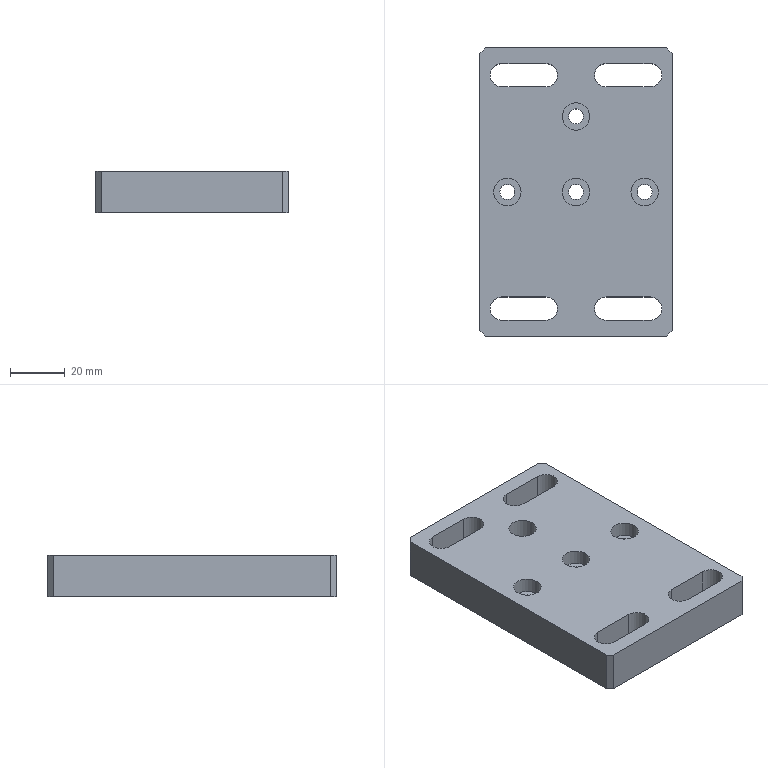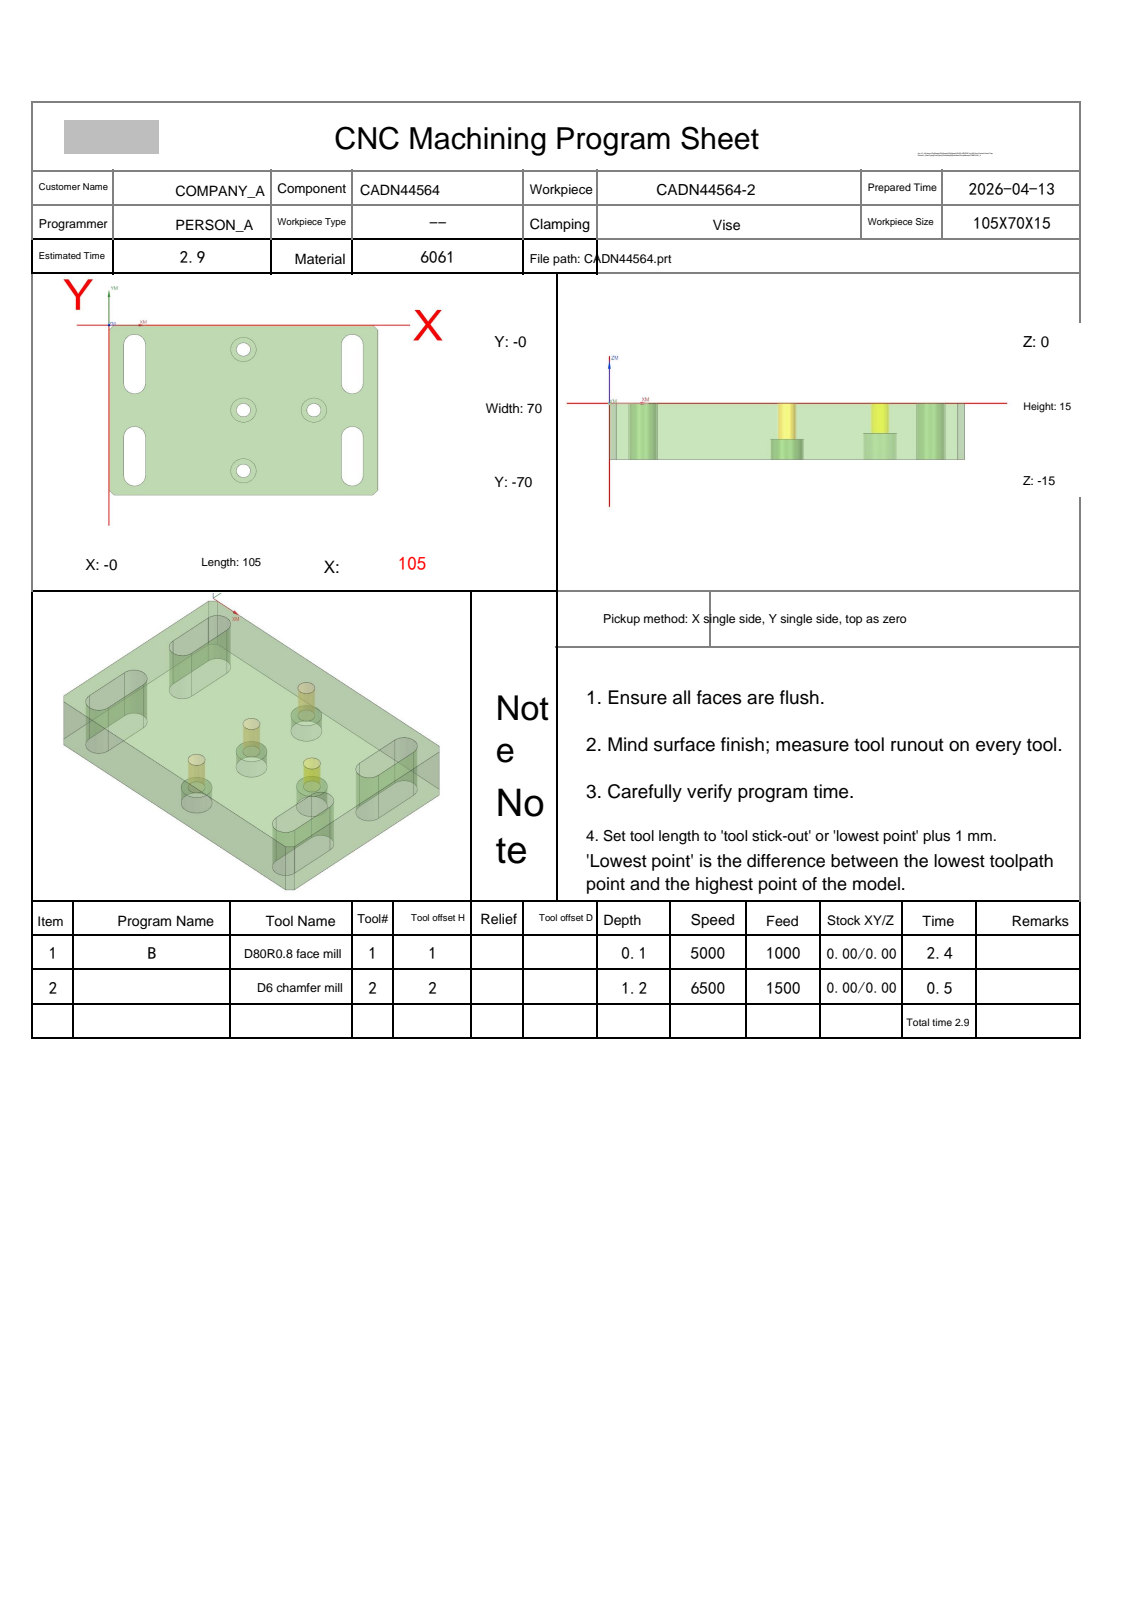NC program | NX | posted by the shop | part box 70 x 105 x 15 mm
Whole program:
%
O0001
(Machine time: 3.19 MIN)
(===Total Tool:2===)
(T1=D80R0.8 face mill D=80.  R=0.8  D-  H01 Z=0.    )
(T2=D6 chamfer mill   D=6.   R=0.   D-  H02 Z=-1.2  )
G80 G90 G17 G49 G40
G91 G28 Z0
M01
N1 T01 M06
(D80R0.8 face mill  D=80. R=0.8 H=01 ce=0.00 di=0.10)
G00 G90 G54 X-45. Y-35. M03 S5000
G43 H01 Z20.
M08
Z6.51
G01 Z4.51 F1000.
X-40.
X145.
X150.
Z6.51
G00 Z8.
X-45.
Z6.02
G01 Z4.02
X-40.
X145.
X150.
Z6.02
G00 Z7.51
X-45.
Z5.53
G01 Z3.53
X-40.
X145.
X150.
Z5.53
G00 Z7.02
X-45.
Z5.04
G01 Z3.04
X-40.
X145.
X150.
Z5.04
G00 Z6.53
X-45.
Z4.55
G01 Z2.55
X-40.
X145.
X150.
Z4.55
G00 Z6.04
X-45.
Z4.06
G01 Z2.06
X-40.
X145.
X150.
Z4.06
G00 Z5.55
X-45.
Z3.57
G01 Z1.57
X-40.
X145.
X150.
Z3.57
G00 Z5.06
X-45.
Z3.08
G01 Z1.08
X-40.
X145.
X150.
Z3.08
G00 Z4.57
X-45.
Z2.59
G01 Z.59
X-40.
X145.
X150.
Z2.59
G00 Z4.08
X-45.
Z2.1
G01 Z.1
X-40.
X145.
X150.
Z2.1
G00 Z20.
G00 G90 X-45. Y-35. M03 S5000
Z20.
Z2.
G01 Z0.0 F1000.
X-40.
X145.
X150.
Z2.
G00 Z20.
G91 G28 Z0.0
M05
M09
G91 G28 Z0.0
M01
N2 T02 M06
(D6 chamfer mill  D=6. R=0. H=02 ce=0.00 di=0.00)
G00 G90 G54 X52.114 Y1.227 M03 S6500
G43 H02 Z20.
M08
Z.172
G01 Z-1.2 F1500.
G03 X52.4 Y1.027 I1.286 J1.532
G01 X52.446 Y.997
X52.5 Y1.
X103.
X103.259 Y.966
X103.5 Y.866
X103.707 Y.707
X105.707 Y-1.293
X105.866 Y-1.5
X105.966 Y-1.741
X106. Y-2.
Y-68.
X105.966 Y-68.259
X105.866 Y-68.5
X105.707 Y-68.707
X103.707 Y-70.707
X103.5 Y-70.866
X103.259 Y-70.966
X103. Y-71.
X2.
X1.741 Y-70.966
X1.5 Y-70.866
X1.293 Y-70.707
X-.707 Y-68.707
X-.866 Y-68.5
X-.966 Y-68.259
X-1. Y-68.
Y-2.
X-.966 Y-1.741
X-.866 Y-1.5
X-.707 Y-1.293
X1.293 Y.707
X1.5 Y.866
X1.741 Y.966
X2. Y1.
X52.5
X52.554 Y.997
X52.6 Y1.027
G03 X52.886 Y1.227 I-1. J1.732
G01 Z.172
G00 Z10.
X91.977 Y-53.614
Z.172
G01 Z-1.2
G03 X91.777 Y-53.9 I1.532 J-1.286
G01 X91.747 Y-53.946
X91.75 Y-54.
Y-62.
G03 X95. Y-65.25 I3.25 J0.0
X98.25 Y-62. I0.0 J3.25
G01 Y-46.
G03 X95. Y-42.75 I-3.25 J0.0
X91.75 Y-46. I0.0 J-3.25
G01 Y-54.
X91.747 Y-54.054
X91.777 Y-54.1
G03 X91.977 Y-54.386 I1.732 J1.
G01 Z.172
G00 Z10.
X79.593 Y-36.565
Z.27
G01 Z-1.2
G03 X79.898 Y-36.734 I1.118 J1.658
G01 X79.946 Y-36.759
X80. Y-36.75
G03 X81.75 Y-35. I0.0 J1.75
X80. Y-33.25 I-1.75 J0.0
X78.25 Y-35. I0.0 J-1.75
X80. Y-36.75 I1.75 J0.0
G01 X80.054 Y-36.759
X80.102 Y-36.734
G03 X80.407 Y-36.565 I-.813 J1.827
G01 Z.27
G00 Z10.
X91.977 Y-15.614
Z.172
G01 Z-1.2
G03 X91.777 Y-15.9 I1.532 J-1.286
G01 X91.747 Y-15.946
X91.75 Y-16.
Y-24.
G03 X95. Y-27.25 I3.25 J0.0
X98.25 Y-24. I0.0 J3.25
G01 Y-8.
G03 X95. Y-4.75 I-3.25 J0.0
X91.75 Y-8. I0.0 J-3.25
G01 Y-16.
X91.747 Y-16.054
X91.777 Y-16.1
G03 X91.977 Y-16.386 I1.732 J1.
G01 Z.172
G00 Z10.
X52.093 Y-11.565
Z.27
G01 Z-1.2
G03 X52.398 Y-11.734 I1.118 J1.658
G01 X52.446 Y-11.759
X52.5 Y-11.75
G03 X54.25 Y-10. I0.0 J1.75
X52.5 Y-8.25 I-1.75 J0.0
X50.75 Y-10. I0.0 J-1.75
X52.5 Y-11.75 I1.75 J0.0
G01 X52.554 Y-11.759
X52.602 Y-11.734
G03 X52.907 Y-11.565 I-.813 J1.827
G01 Z.27
G00 Z10.
X52.093 Y-36.565
Z.27
G01 Z-1.2
G03 X52.398 Y-36.734 I1.118 J1.658
G01 X52.446 Y-36.759
X52.5 Y-36.75
G03 X54.25 Y-35. I0.0 J1.75
X52.5 Y-33.25 I-1.75 J0.0
X50.75 Y-35. I0.0 J-1.75
X52.5 Y-36.75 I1.75 J0.0
G01 X52.554 Y-36.759
X52.602 Y-36.734
G03 X52.907 Y-36.565 I-.813 J1.827
G01 Z.27
G00 Z10.
X52.093 Y-61.565
Z.27
G01 Z-1.2
G03 X52.398 Y-61.734 I1.118 J1.658
G01 X52.446 Y-61.759
X52.5 Y-61.75
G03 X54.25 Y-60. I0.0 J1.75
X52.5 Y-58.25 I-1.75 J0.0
X50.75 Y-60. I0.0 J-1.75
X52.5 Y-61.75 I1.75 J0.0
G01 X52.554 Y-61.759
X52.602 Y-61.734
G03 X52.907 Y-61.565 I-.813 J1.827
G01 Z.27
G00 Z10.
X13.023 Y-54.386
Z.172
G01 Z-1.2
G03 X13.223 Y-54.1 I-1.532 J1.286
G01 X13.253 Y-54.054
X13.25 Y-54.
Y-46.
G03 X10. Y-42.75 I-3.25 J0.0
X6.75 Y-46. I0.0 J-3.25
G01 Y-62.
G03 X10. Y-65.25 I3.25 J0.0
X13.25 Y-62. I0.0 J3.25
G01 Y-54.
X13.253 Y-53.946
X13.223 Y-53.9
G03 X13.023 Y-53.614 I-1.732 J-1.
G01 Z.172
G00 Z10.
Y-16.386
Z.172
G01 Z-1.2
G03 X13.223 Y-16.1 I-1.532 J1.286
G01 X13.253 Y-16.054
X13.25 Y-16.
Y-8.
G03 X10. Y-4.75 I-3.25 J0.0
X6.75 Y-8. I0.0 J-3.25
G01 Y-24.
G03 X10. Y-27.25 I3.25 J0.0
X13.25 Y-24. I0.0 J3.25
G01 Y-16.
X13.253 Y-15.946
X13.223 Y-15.9
G03 X13.023 Y-15.614 I-1.732 J-1.
G01 Z.172
G00 Z20.
M05
M09
G91 G28 Z0.0
G91 G28 Y0.0
M30
%